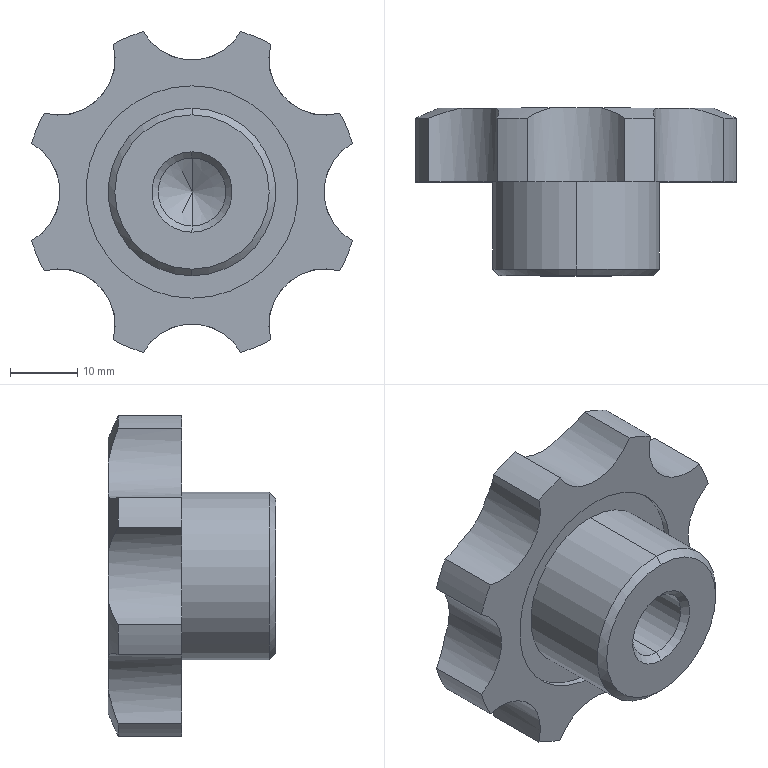Part | SolidWorks | features BaseBody 1 | 1 solid | 46 faces | box 47.841 x 25 x 47.841 mm | volume 21610 mm3 | cylinder 26 | cone 14 | plane 6 | commonest cylinder face diameters 16.667 x8 50 x8 25 x4 31.667 x4 10.106 x2
STEP:
#1=CARTESIAN_POINT('',(0.,0.947,-5.053));
#2=VERTEX_POINT('',#1);
#3=CARTESIAN_POINT('',(-0.000000001,0.947,5.053));
#4=VERTEX_POINT('',#3);
#5=CARTESIAN_POINT('',(0.,0.947,0.));
#6=DIRECTION('',(0.,-1.,0.));
#7=DIRECTION('',(0.,0.,1.));
#8=AXIS2_PLACEMENT_3D('',#5,#6,#7);
#9=CIRCLE('',#8,5.053);
#10=EDGE_CURVE('',#2,#4,#9,.T.);
#11=ORIENTED_EDGE('',*,*,#10,.F.);
#12=CARTESIAN_POINT('',(0.,0.,-6.));
#13=VERTEX_POINT('',#12);
#14=CARTESIAN_POINT('',(0.,0.,-6.));
#15=DIRECTION('',(0.,-0.7071,-0.7071));
#16=VECTOR('',#15,1000.);
#17=LINE('',#14,#16);
#18=EDGE_CURVE('',#2,#13,#17,.T.);
#19=ORIENTED_EDGE('',*,*,#18,.T.);
#20=CARTESIAN_POINT('',(0.,0.,6.));
#21=VERTEX_POINT('',#20);
#22=CARTESIAN_POINT('',(0.,0.,0.));
#23=DIRECTION('',(0.,-1.,0.));
#24=DIRECTION('',(0.,0.,-1.));
#25=AXIS2_PLACEMENT_3D('',#22,#23,#24);
#26=CIRCLE('',#25,6.);
#27=EDGE_CURVE('',#13,#21,#26,.T.);
#28=ORIENTED_EDGE('',*,*,#27,.T.);
#29=CARTESIAN_POINT('',(0.,0.,6.));
#30=DIRECTION('',(0.,-0.7071,0.7071));
#31=VECTOR('',#30,1000.);
#32=LINE('',#29,#31);
#33=EDGE_CURVE('',#4,#21,#32,.T.);
#34=ORIENTED_EDGE('',*,*,#33,.F.);
#35=EDGE_LOOP('',(#11,#19,#28,#34));
#36=FACE_OUTER_BOUND('',#35,.T.);
#37=CARTESIAN_POINT('',(0.,0.,0.));
#38=DIRECTION('',(0.,-1.,0.));
#39=DIRECTION('',(0.,0.,1.));
#40=AXIS2_PLACEMENT_3D('',#37,#38,#39);
#41=CONICAL_SURFACE('',#40,6.,0.7854);
#42=ADVANCED_FACE('',(#36),#41,.F.);
#43=CARTESIAN_POINT('',(0.,15.047,-5.053));
#44=VERTEX_POINT('',#43);
#45=CARTESIAN_POINT('',(0.,15.047,5.053));
#46=VERTEX_POINT('',#45);
#47=CARTESIAN_POINT('',(0.,15.047,0.));
#48=DIRECTION('',(0.,-1.,0.));
#49=DIRECTION('',(0.,0.,1.));
#50=AXIS2_PLACEMENT_3D('',#47,#48,#49);
#51=CIRCLE('',#50,5.053);
#52=EDGE_CURVE('',#44,#46,#51,.T.);
#53=ORIENTED_EDGE('',*,*,#52,.F.);
#54=CARTESIAN_POINT('',(0.,0.,-5.053));
#55=DIRECTION('',(0.,-1.,0.));
#56=VECTOR('',#55,1000.);
#57=LINE('',#54,#56);
#58=EDGE_CURVE('',#44,#2,#57,.T.);
#59=ORIENTED_EDGE('',*,*,#58,.T.);
#60=ORIENTED_EDGE('',*,*,#10,.T.);
#61=CARTESIAN_POINT('',(0.,0.,5.053));
#62=DIRECTION('',(0.,-1.,0.));
#63=VECTOR('',#62,1000.);
#64=LINE('',#61,#63);
#65=EDGE_CURVE('',#46,#4,#64,.T.);
#66=ORIENTED_EDGE('',*,*,#65,.F.);
#67=EDGE_LOOP('',(#53,#59,#60,#66));
#68=FACE_OUTER_BOUND('',#67,.T.);
#69=CARTESIAN_POINT('',(0.,0.,0.));
#70=DIRECTION('',(0.,-1.,0.));
#71=DIRECTION('',(0.,0.,1.));
#72=AXIS2_PLACEMENT_3D('',#69,#70,#71);
#73=CYLINDRICAL_SURFACE('',#72,5.053);
#74=ADVANCED_FACE('',(#68),#73,.F.);
#75=CARTESIAN_POINT('',(0.,17.964,0.));
#76=VERTEX_POINT('',#75);
#77=CARTESIAN_POINT('',(0.,15.047,5.053));
#78=DIRECTION('',(0.,-0.5,0.866));
#79=VECTOR('',#78,1000.);
#80=LINE('',#77,#79);
#81=EDGE_CURVE('',#76,#46,#80,.T.);
#82=ORIENTED_EDGE('',*,*,#81,.F.);
#83=CARTESIAN_POINT('',(0.,15.047,-5.053));
#84=DIRECTION('',(0.,-0.5,-0.866));
#85=VECTOR('',#84,1000.);
#86=LINE('',#83,#85);
#87=EDGE_CURVE('',#76,#44,#86,.T.);
#88=ORIENTED_EDGE('',*,*,#87,.T.);
#89=ORIENTED_EDGE('',*,*,#52,.T.);
#90=EDGE_LOOP('',(#82,#88,#89));
#91=FACE_OUTER_BOUND('',#90,.T.);
#92=CARTESIAN_POINT('',(0.,15.047,0.));
#93=DIRECTION('',(0.,-1.,0.));
#94=DIRECTION('',(0.,0.,1.));
#95=AXIS2_PLACEMENT_3D('',#92,#93,#94);
#96=CONICAL_SURFACE('',#95,5.053,1.047);
#97=ADVANCED_FACE('',(#91),#96,.F.);
#98=CARTESIAN_POINT('',(0.,0.,11.5));
#99=VERTEX_POINT('',#98);
#100=CARTESIAN_POINT('',(0.,0.,-11.5));
#101=VERTEX_POINT('',#100);
#102=CARTESIAN_POINT('',(0.,0.,0.));
#103=DIRECTION('',(0.,-1.,0.));
#104=DIRECTION('',(0.,0.,1.));
#105=AXIS2_PLACEMENT_3D('',#102,#103,#104);
#106=CIRCLE('',#105,11.5);
#107=EDGE_CURVE('',#99,#101,#106,.T.);
#108=ORIENTED_EDGE('',*,*,#107,.F.);
#109=CARTESIAN_POINT('',(0.000000015,1.,12.5));
#110=VERTEX_POINT('',#109);
#111=CARTESIAN_POINT('',(0.,1.,12.5));
#112=DIRECTION('',(0.,0.7071,0.7071));
#113=VECTOR('',#112,1000.);
#114=LINE('',#111,#113);
#115=EDGE_CURVE('',#99,#110,#114,.T.);
#116=ORIENTED_EDGE('',*,*,#115,.T.);
#117=CARTESIAN_POINT('',(-0.000000015,1.,-12.5));
#118=VERTEX_POINT('',#117);
#119=CARTESIAN_POINT('',(0.,1.,0.));
#120=DIRECTION('',(0.,-1.,0.));
#121=DIRECTION('',(0.,0.,-1.));
#122=AXIS2_PLACEMENT_3D('',#119,#120,#121);
#123=CIRCLE('',#122,12.5);
#124=EDGE_CURVE('',#110,#118,#123,.T.);
#125=ORIENTED_EDGE('',*,*,#124,.T.);
#126=CARTESIAN_POINT('',(0.,1.,-12.5));
#127=DIRECTION('',(0.,0.7071,-0.7071));
#128=VECTOR('',#127,1000.);
#129=LINE('',#126,#128);
#130=EDGE_CURVE('',#101,#118,#129,.T.);
#131=ORIENTED_EDGE('',*,*,#130,.F.);
#132=EDGE_LOOP('',(#108,#116,#125,#131));
#133=FACE_OUTER_BOUND('',#132,.T.);
#134=CARTESIAN_POINT('',(0.,1.,0.));
#135=DIRECTION('',(0.,1.,0.));
#136=DIRECTION('',(0.,0.,-1.));
#137=AXIS2_PLACEMENT_3D('',#134,#135,#136);
#138=CONICAL_SURFACE('',#137,12.5,0.7854);
#139=ADVANCED_FACE('',(#133),#138,.T.);
#140=CARTESIAN_POINT('',(0.000000015,15.,12.5));
#141=VERTEX_POINT('',#140);
#142=CARTESIAN_POINT('',(-0.000000015,15.,-12.5));
#143=VERTEX_POINT('',#142);
#144=CARTESIAN_POINT('',(0.,15.,0.));
#145=DIRECTION('',(0.,-1.,0.));
#146=DIRECTION('',(0.,0.,-1.));
#147=AXIS2_PLACEMENT_3D('',#144,#145,#146);
#148=CIRCLE('',#147,12.5);
#149=EDGE_CURVE('',#141,#143,#148,.T.);
#150=ORIENTED_EDGE('',*,*,#149,.T.);
#151=CARTESIAN_POINT('',(-0.000000015,0.,-12.5));
#152=DIRECTION('',(0.,-1.,0.));
#153=VECTOR('',#152,1000.);
#154=LINE('',#151,#153);
#155=EDGE_CURVE('',#143,#118,#154,.T.);
#156=ORIENTED_EDGE('',*,*,#155,.T.);
#157=ORIENTED_EDGE('',*,*,#124,.F.);
#158=CARTESIAN_POINT('',(0.000000015,0.,12.5));
#159=DIRECTION('',(0.,-1.,0.));
#160=VECTOR('',#159,1000.);
#161=LINE('',#158,#160);
#162=EDGE_CURVE('',#141,#110,#161,.T.);
#163=ORIENTED_EDGE('',*,*,#162,.F.);
#164=EDGE_LOOP('',(#150,#156,#157,#163));
#165=FACE_OUTER_BOUND('',#164,.T.);
#166=CARTESIAN_POINT('',(0.,0.,0.));
#167=DIRECTION('',(0.,-1.,0.));
#168=DIRECTION('',(0.000000001,0.,1.));
#169=AXIS2_PLACEMENT_3D('',#166,#167,#168);
#170=CYLINDRICAL_SURFACE('',#169,12.5);
#171=ADVANCED_FACE('',(#165),#170,.T.);
#172=CARTESIAN_POINT('',(0.,15.,-15.833));
#173=VERTEX_POINT('',#172);
#174=CARTESIAN_POINT('',(0.,15.,15.833));
#175=VERTEX_POINT('',#174);
#176=CARTESIAN_POINT('',(0.,15.,0.));
#177=DIRECTION('',(0.,-1.,0.));
#178=DIRECTION('',(0.,0.,1.));
#179=AXIS2_PLACEMENT_3D('',#176,#177,#178);
#180=CIRCLE('',#179,15.833);
#181=EDGE_CURVE('',#173,#175,#180,.T.);
#182=ORIENTED_EDGE('',*,*,#181,.F.);
#183=CARTESIAN_POINT('',(0.,14.,-15.833));
#184=VERTEX_POINT('',#183);
#185=CARTESIAN_POINT('',(0.,0.,-15.833));
#186=DIRECTION('',(0.,-1.,0.));
#187=VECTOR('',#186,1000.);
#188=LINE('',#185,#187);
#189=EDGE_CURVE('',#173,#184,#188,.T.);
#190=ORIENTED_EDGE('',*,*,#189,.T.);
#191=CARTESIAN_POINT('',(0.,14.,15.833));
#192=VERTEX_POINT('',#191);
#193=CARTESIAN_POINT('',(0.,14.,0.));
#194=DIRECTION('',(0.,-1.,0.));
#195=DIRECTION('',(0.,0.,-1.));
#196=AXIS2_PLACEMENT_3D('',#193,#194,#195);
#197=CIRCLE('',#196,15.833);
#198=EDGE_CURVE('',#184,#192,#197,.T.);
#199=ORIENTED_EDGE('',*,*,#198,.T.);
#200=CARTESIAN_POINT('',(0.,0.,15.833));
#201=DIRECTION('',(0.,-1.,0.));
#202=VECTOR('',#201,1000.);
#203=LINE('',#200,#202);
#204=EDGE_CURVE('',#175,#192,#203,.T.);
#205=ORIENTED_EDGE('',*,*,#204,.F.);
#206=EDGE_LOOP('',(#182,#190,#199,#205));
#207=FACE_OUTER_BOUND('',#206,.T.);
#208=CARTESIAN_POINT('',(0.,0.,0.));
#209=DIRECTION('',(0.,-1.,0.));
#210=DIRECTION('',(0.,0.,1.));
#211=AXIS2_PLACEMENT_3D('',#208,#209,#210);
#212=CYLINDRICAL_SURFACE('',#211,15.833);
#213=ADVANCED_FACE('',(#207),#212,.F.);
#214=CARTESIAN_POINT('',(0.,25.,-15.833));
#215=VERTEX_POINT('',#214);
#216=CARTESIAN_POINT('',(0.,25.,15.833));
#217=VERTEX_POINT('',#216);
#218=CARTESIAN_POINT('',(0.,25.,0.));
#219=DIRECTION('',(0.,-1.,0.));
#220=DIRECTION('',(0.,0.,1.));
#221=AXIS2_PLACEMENT_3D('',#218,#219,#220);
#222=CIRCLE('',#221,15.833);
#223=EDGE_CURVE('',#215,#217,#222,.T.);
#224=ORIENTED_EDGE('',*,*,#223,.F.);
#225=CARTESIAN_POINT('',(0.,24.,-15.833));
#226=VERTEX_POINT('',#225);
#227=CARTESIAN_POINT('',(0.,0.,-15.833));
#228=DIRECTION('',(0.,-1.,0.));
#229=VECTOR('',#228,1000.);
#230=LINE('',#227,#229);
#231=EDGE_CURVE('',#215,#226,#230,.T.);
#232=ORIENTED_EDGE('',*,*,#231,.T.);
#233=CARTESIAN_POINT('',(0.,24.,15.833));
#234=VERTEX_POINT('',#233);
#235=CARTESIAN_POINT('',(0.,24.,0.));
#236=DIRECTION('',(0.,-1.,0.));
#237=DIRECTION('',(0.,0.,-1.));
#238=AXIS2_PLACEMENT_3D('',#235,#236,#237);
#239=CIRCLE('',#238,15.833);
#240=EDGE_CURVE('',#226,#234,#239,.T.);
#241=ORIENTED_EDGE('',*,*,#240,.T.);
#242=CARTESIAN_POINT('',(0.,0.,15.833));
#243=DIRECTION('',(0.,-1.,0.));
#244=VECTOR('',#243,1000.);
#245=LINE('',#242,#244);
#246=EDGE_CURVE('',#217,#234,#245,.T.);
#247=ORIENTED_EDGE('',*,*,#246,.F.);
#248=EDGE_LOOP('',(#224,#232,#241,#247));
#249=FACE_OUTER_BOUND('',#248,.T.);
#250=CARTESIAN_POINT('',(0.,0.,0.));
#251=DIRECTION('',(0.,-1.,0.));
#252=DIRECTION('',(0.,0.,1.));
#253=AXIS2_PLACEMENT_3D('',#250,#251,#252);
#254=CYLINDRICAL_SURFACE('',#253,15.833);
#255=ADVANCED_FACE('',(#249),#254,.F.);
#256=CARTESIAN_POINT('',(0.,25.,12.5));
#257=VERTEX_POINT('',#256);
#258=CARTESIAN_POINT('',(0.,25.,-12.5));
#259=VERTEX_POINT('',#258);
#260=CARTESIAN_POINT('',(0.,25.,0.));
#261=DIRECTION('',(0.,-1.,0.));
#262=DIRECTION('',(0.,0.,-1.));
#263=AXIS2_PLACEMENT_3D('',#260,#261,#262);
#264=CIRCLE('',#263,12.5);
#265=EDGE_CURVE('',#257,#259,#264,.T.);
#266=ORIENTED_EDGE('',*,*,#265,.T.);
#267=CARTESIAN_POINT('',(0.,24.,-12.5));
#268=VERTEX_POINT('',#267);
#269=CARTESIAN_POINT('',(0.,0.,-12.5));
#270=DIRECTION('',(0.,-1.,0.));
#271=VECTOR('',#270,1000.);
#272=LINE('',#269,#271);
#273=EDGE_CURVE('',#259,#268,#272,.T.);
#274=ORIENTED_EDGE('',*,*,#273,.T.);
#275=CARTESIAN_POINT('',(-0.000000015,24.,12.5));
#276=VERTEX_POINT('',#275);
#277=CARTESIAN_POINT('',(0.,24.,0.));
#278=DIRECTION('',(0.,-1.,0.));
#279=DIRECTION('',(-0.000000001,0.,1.));
#280=AXIS2_PLACEMENT_3D('',#277,#278,#279);
#281=CIRCLE('',#280,12.5);
#282=EDGE_CURVE('',#276,#268,#281,.T.);
#283=ORIENTED_EDGE('',*,*,#282,.F.);
#284=CARTESIAN_POINT('',(0.,0.,12.5));
#285=DIRECTION('',(0.,-1.,0.));
#286=VECTOR('',#285,1000.);
#287=LINE('',#284,#286);
#288=EDGE_CURVE('',#257,#276,#287,.T.);
#289=ORIENTED_EDGE('',*,*,#288,.F.);
#290=EDGE_LOOP('',(#266,#274,#283,#289));
#291=FACE_OUTER_BOUND('',#290,.T.);
#292=CARTESIAN_POINT('',(0.,0.,0.));
#293=DIRECTION('',(0.,-1.,0.));
#294=DIRECTION('',(0.,0.,1.));
#295=AXIS2_PLACEMENT_3D('',#292,#293,#294);
#296=CYLINDRICAL_SURFACE('',#295,12.5);
#297=ADVANCED_FACE('',(#291),#296,.T.);
#298=CARTESIAN_POINT('',(-11.895,25.,-17.159));
#299=VERTEX_POINT('',#298);
#300=CARTESIAN_POINT('',(-11.776,23.5,-22.053));
#301=VERTEX_POINT('',#300);
#302=CARTESIAN_POINT('',(-11.895,25.,-17.159));
#303=CARTESIAN_POINT('',(-11.631,24.818,-17.949));
#304=CARTESIAN_POINT('',(-11.486,24.587,-18.784));
#305=CARTESIAN_POINT('',(-11.449,24.071,-20.447));
#306=CARTESIAN_POINT('',(-11.558,23.787,-21.275));
#307=CARTESIAN_POINT('',(-11.776,23.5,-22.053));
#308=B_SPLINE_CURVE_WITH_KNOTS('',3,(#302,#303,#304,#305,#306,#307),.UNSPECIFIED.,.F.,.F.,(4,2,4),(0.,0.5,1.),.UNSPECIFIED.);
#309=EDGE_CURVE('',#299,#301,#308,.T.);
#310=ORIENTED_EDGE('',*,*,#309,.F.);
#311=CARTESIAN_POINT('',(-3.722,25.,-20.544));
#312=VERTEX_POINT('',#311);
#313=CARTESIAN_POINT('',(0.,25.,0.));
#314=DIRECTION('',(0.,-1.,0.));
#315=DIRECTION('',(-0.5697,0.,-0.8218));
#316=AXIS2_PLACEMENT_3D('',#313,#314,#315);
#317=CIRCLE('',#316,20.879);
#318=EDGE_CURVE('',#299,#312,#317,.T.);
#319=ORIENTED_EDGE('',*,*,#318,.T.);
#320=CARTESIAN_POINT('',(-7.267,23.5,-23.921));
#321=VERTEX_POINT('',#320);
#322=CARTESIAN_POINT('',(-7.267,23.5,-23.921));
#323=CARTESIAN_POINT('',(-6.875,23.784,-23.223));
#324=CARTESIAN_POINT('',(-6.369,24.068,-22.562));
#325=CARTESIAN_POINT('',(-5.167,24.585,-21.409));
#326=CARTESIAN_POINT('',(-4.471,24.818,-20.918));
#327=CARTESIAN_POINT('',(-3.722,25.,-20.544));
#328=B_SPLINE_CURVE_WITH_KNOTS('',3,(#322,#323,#324,#325,#326,#327),.UNSPECIFIED.,.F.,.F.,(4,2,4),(0.,0.5,1.),.UNSPECIFIED.);
#329=EDGE_CURVE('',#321,#312,#328,.T.);
#330=ORIENTED_EDGE('',*,*,#329,.F.);
#331=CARTESIAN_POINT('',(0.,23.5,0.));
#332=DIRECTION('',(0.,-1.,0.));
#333=DIRECTION('',(-0.2907,0.,-0.9568));
#334=AXIS2_PLACEMENT_3D('',#331,#332,#333);
#335=CIRCLE('',#334,25.);
#336=EDGE_CURVE('',#301,#321,#335,.T.);
#337=ORIENTED_EDGE('',*,*,#336,.F.);
#338=EDGE_LOOP('',(#310,#319,#330,#337));
#339=FACE_OUTER_BOUND('',#338,.T.);
#340=CARTESIAN_POINT('',(0.,23.5,0.));
#341=DIRECTION('',(0.,-1.,0.));
#342=DIRECTION('',(-0.5697,0.,-0.8218));
#343=AXIS2_PLACEMENT_3D('',#340,#341,#342);
#344=CONICAL_SURFACE('',#343,25.,1.222);
#345=ADVANCED_FACE('',(#339),#344,.T.);
#346=CARTESIAN_POINT('',(-22.053,23.5,-11.776));
#347=VERTEX_POINT('',#346);
#348=CARTESIAN_POINT('',(-17.159,25.,-11.895));
#349=VERTEX_POINT('',#348);
#350=CARTESIAN_POINT('',(-22.053,23.5,-11.776));
#351=CARTESIAN_POINT('',(-21.283,23.784,-11.56));
#352=CARTESIAN_POINT('',(-20.457,24.068,-11.45));
#353=CARTESIAN_POINT('',(-18.792,24.585,-11.485));
#354=CARTESIAN_POINT('',(-17.953,24.818,-11.63));
#355=CARTESIAN_POINT('',(-17.159,25.,-11.895));
#356=B_SPLINE_CURVE_WITH_KNOTS('',3,(#350,#351,#352,#353,#354,#355),.UNSPECIFIED.,.F.,.F.,(4,2,4),(0.,0.5,1.),.UNSPECIFIED.);
#357=EDGE_CURVE('',#347,#349,#356,.T.);
#358=ORIENTED_EDGE('',*,*,#357,.F.);
#359=CARTESIAN_POINT('',(-23.921,23.5,-7.267));
#360=VERTEX_POINT('',#359);
#361=CARTESIAN_POINT('',(0.,23.5,0.));
#362=DIRECTION('',(0.,-1.,0.));
#363=DIRECTION('',(-0.8821,0.,-0.471));
#364=AXIS2_PLACEMENT_3D('',#361,#362,#363);
#365=CIRCLE('',#364,25.);
#366=EDGE_CURVE('',#360,#347,#365,.T.);
#367=ORIENTED_EDGE('',*,*,#366,.F.);
#368=CARTESIAN_POINT('',(-20.544,25.,-3.722));
#369=VERTEX_POINT('',#368);
#370=CARTESIAN_POINT('',(-20.544,25.,-3.722));
#371=CARTESIAN_POINT('',(-20.916,24.818,-4.467));
#372=CARTESIAN_POINT('',(-21.404,24.587,-5.16));
#373=CARTESIAN_POINT('',(-22.554,24.071,-6.362));
#374=CARTESIAN_POINT('',(-23.216,23.787,-6.871));
#375=CARTESIAN_POINT('',(-23.921,23.5,-7.267));
#376=B_SPLINE_CURVE_WITH_KNOTS('',3,(#370,#371,#372,#373,#374,#375),.UNSPECIFIED.,.F.,.F.,(4,2,4),(0.,0.5,1.),.UNSPECIFIED.);
#377=EDGE_CURVE('',#369,#360,#376,.T.);
#378=ORIENTED_EDGE('',*,*,#377,.F.);
#379=CARTESIAN_POINT('',(0.,25.,0.));
#380=DIRECTION('',(0.,-1.,0.));
#381=DIRECTION('',(-0.984,0.,-0.1783));
#382=AXIS2_PLACEMENT_3D('',#379,#380,#381);
#383=CIRCLE('',#382,20.879);
#384=EDGE_CURVE('',#369,#349,#383,.T.);
#385=ORIENTED_EDGE('',*,*,#384,.T.);
#386=EDGE_LOOP('',(#358,#367,#378,#385));
#387=FACE_OUTER_BOUND('',#386,.T.);
#388=CARTESIAN_POINT('',(0.,23.5,0.));
#389=DIRECTION('',(0.,-1.,0.));
#390=DIRECTION('',(-0.984,0.,-0.1783));
#391=AXIS2_PLACEMENT_3D('',#388,#389,#390);
#392=CONICAL_SURFACE('',#391,25.,1.222);
#393=ADVANCED_FACE('',(#387),#392,.T.);
#394=CARTESIAN_POINT('',(3.722,25.,-20.544));
#395=VERTEX_POINT('',#394);
#396=CARTESIAN_POINT('',(7.267,23.5,-23.921));
#397=VERTEX_POINT('',#396);
#398=CARTESIAN_POINT('',(3.722,25.,-20.544));
#399=CARTESIAN_POINT('',(4.467,24.818,-20.916));
#400=CARTESIAN_POINT('',(5.16,24.587,-21.404));
#401=CARTESIAN_POINT('',(6.362,24.071,-22.554));
#402=CARTESIAN_POINT('',(6.871,23.787,-23.216));
#403=CARTESIAN_POINT('',(7.267,23.5,-23.921));
#404=B_SPLINE_CURVE_WITH_KNOTS('',3,(#398,#399,#400,#401,#402,#403),.UNSPECIFIED.,.F.,.F.,(4,2,4),(0.,0.5,1.),.UNSPECIFIED.);
#405=EDGE_CURVE('',#395,#397,#404,.T.);
#406=ORIENTED_EDGE('',*,*,#405,.F.);
#407=CARTESIAN_POINT('',(11.895,25.,-17.159));
#408=VERTEX_POINT('',#407);
#409=CARTESIAN_POINT('',(0.,25.,0.));
#410=DIRECTION('',(0.,-1.,0.));
#411=DIRECTION('',(0.1783,0.,-0.984));
#412=AXIS2_PLACEMENT_3D('',#409,#410,#411);
#413=CIRCLE('',#412,20.879);
#414=EDGE_CURVE('',#395,#408,#413,.T.);
#415=ORIENTED_EDGE('',*,*,#414,.T.);
#416=CARTESIAN_POINT('',(11.776,23.5,-22.053));
#417=VERTEX_POINT('',#416);
#418=CARTESIAN_POINT('',(11.776,23.5,-22.053));
#419=CARTESIAN_POINT('',(11.56,23.784,-21.283));
#420=CARTESIAN_POINT('',(11.45,24.068,-20.457));
#421=CARTESIAN_POINT('',(11.485,24.585,-18.792));
#422=CARTESIAN_POINT('',(11.63,24.818,-17.953));
#423=CARTESIAN_POINT('',(11.895,25.,-17.159));
#424=B_SPLINE_CURVE_WITH_KNOTS('',3,(#418,#419,#420,#421,#422,#423),.UNSPECIFIED.,.F.,.F.,(4,2,4),(0.,0.5,1.),.UNSPECIFIED.);
#425=EDGE_CURVE('',#417,#408,#424,.T.);
#426=ORIENTED_EDGE('',*,*,#425,.F.);
#427=CARTESIAN_POINT('',(0.,23.5,0.));
#428=DIRECTION('',(0.,-1.,0.));
#429=DIRECTION('',(0.471,0.,-0.8821));
#430=AXIS2_PLACEMENT_3D('',#427,#428,#429);
#431=CIRCLE('',#430,25.);
#432=EDGE_CURVE('',#397,#417,#431,.T.);
#433=ORIENTED_EDGE('',*,*,#432,.F.);
#434=EDGE_LOOP('',(#406,#415,#426,#433));
#435=FACE_OUTER_BOUND('',#434,.T.);
#436=CARTESIAN_POINT('',(0.,23.5,0.));
#437=DIRECTION('',(0.,-1.,0.));
#438=DIRECTION('',(0.1783,0.,-0.984));
#439=AXIS2_PLACEMENT_3D('',#436,#437,#438);
#440=CONICAL_SURFACE('',#439,25.,1.222);
#441=ADVANCED_FACE('',(#435),#440,.T.);
#442=CARTESIAN_POINT('',(17.159,25.,-11.895));
#443=VERTEX_POINT('',#442);
#444=CARTESIAN_POINT('',(22.053,23.5,-11.776));
#445=VERTEX_POINT('',#444);
#446=CARTESIAN_POINT('',(17.159,25.,-11.895));
#447=CARTESIAN_POINT('',(17.949,24.818,-11.631));
#448=CARTESIAN_POINT('',(18.784,24.587,-11.486));
#449=CARTESIAN_POINT('',(20.447,24.071,-11.449));
#450=CARTESIAN_POINT('',(21.275,23.787,-11.558));
#451=CARTESIAN_POINT('',(22.053,23.5,-11.776));
#452=B_SPLINE_CURVE_WITH_KNOTS('',3,(#446,#447,#448,#449,#450,#451),.UNSPECIFIED.,.F.,.F.,(4,2,4),(0.,0.5,1.),.UNSPECIFIED.);
#453=EDGE_CURVE('',#443,#445,#452,.T.);
#454=ORIENTED_EDGE('',*,*,#453,.F.);
#455=CARTESIAN_POINT('',(20.544,25.,-3.722));
#456=VERTEX_POINT('',#455);
#457=CARTESIAN_POINT('',(0.,25.,0.));
#458=DIRECTION('',(0.,-1.,0.));
#459=DIRECTION('',(0.8218,0.,-0.5697));
#460=AXIS2_PLACEMENT_3D('',#457,#458,#459);
#461=CIRCLE('',#460,20.879);
#462=EDGE_CURVE('',#443,#456,#461,.T.);
#463=ORIENTED_EDGE('',*,*,#462,.T.);
#464=CARTESIAN_POINT('',(23.921,23.5,-7.267));
#465=VERTEX_POINT('',#464);
#466=CARTESIAN_POINT('',(23.921,23.5,-7.267));
#467=CARTESIAN_POINT('',(23.223,23.784,-6.875));
#468=CARTESIAN_POINT('',(22.562,24.068,-6.369));
#469=CARTESIAN_POINT('',(21.409,24.585,-5.167));
#470=CARTESIAN_POINT('',(20.918,24.818,-4.471));
#471=CARTESIAN_POINT('',(20.544,25.,-3.722));
#472=B_SPLINE_CURVE_WITH_KNOTS('',3,(#466,#467,#468,#469,#470,#471),.UNSPECIFIED.,.F.,.F.,(4,2,4),(0.,0.5,1.),.UNSPECIFIED.);
#473=EDGE_CURVE('',#465,#456,#472,.T.);
#474=ORIENTED_EDGE('',*,*,#473,.F.);
#475=CARTESIAN_POINT('',(0.,23.5,0.));
#476=DIRECTION('',(0.,-1.,0.));
#477=DIRECTION('',(0.9568,0.,-0.2907));
#478=AXIS2_PLACEMENT_3D('',#475,#476,#477);
#479=CIRCLE('',#478,25.);
#480=EDGE_CURVE('',#445,#465,#479,.T.);
#481=ORIENTED_EDGE('',*,*,#480,.F.);
#482=EDGE_LOOP('',(#454,#463,#474,#481));
#483=FACE_OUTER_BOUND('',#482,.T.);
#484=CARTESIAN_POINT('',(0.,23.5,0.));
#485=DIRECTION('',(0.,-1.,0.));
#486=DIRECTION('',(0.8218,0.,-0.5697));
#487=AXIS2_PLACEMENT_3D('',#484,#485,#486);
#488=CONICAL_SURFACE('',#487,25.,1.222);
#489=ADVANCED_FACE('',(#483),#488,.T.);
#490=CARTESIAN_POINT('',(20.544,25.,3.722));
#491=VERTEX_POINT('',#490);
#492=CARTESIAN_POINT('',(23.921,23.5,7.267));
#493=VERTEX_POINT('',#492);
#494=CARTESIAN_POINT('',(20.544,25.,3.722));
#495=CARTESIAN_POINT('',(20.916,24.818,4.467));
#496=CARTESIAN_POINT('',(21.404,24.587,5.16));
#497=CARTESIAN_POINT('',(22.554,24.071,6.362));
#498=CARTESIAN_POINT('',(23.216,23.787,6.871));
#499=CARTESIAN_POINT('',(23.921,23.5,7.267));
#500=B_SPLINE_CURVE_WITH_KNOTS('',3,(#494,#495,#496,#497,#498,#499),.UNSPECIFIED.,.F.,.F.,(4,2,4),(0.,0.5,1.),.UNSPECIFIED.);
#501=EDGE_CURVE('',#491,#493,#500,.T.);
#502=ORIENTED_EDGE('',*,*,#501,.F.);
#503=CARTESIAN_POINT('',(17.159,25.,11.895));
#504=VERTEX_POINT('',#503);
#505=CARTESIAN_POINT('',(0.,25.,0.));
#506=DIRECTION('',(0.,-1.,0.));
#507=DIRECTION('',(0.984,0.,0.1783));
#508=AXIS2_PLACEMENT_3D('',#505,#506,#507);
#509=CIRCLE('',#508,20.879);
#510=EDGE_CURVE('',#491,#504,#509,.T.);
#511=ORIENTED_EDGE('',*,*,#510,.T.);
#512=CARTESIAN_POINT('',(22.053,23.5,11.776));
#513=VERTEX_POINT('',#512);
#514=CARTESIAN_POINT('',(22.053,23.5,11.776));
#515=CARTESIAN_POINT('',(21.283,23.784,11.56));
#516=CARTESIAN_POINT('',(20.457,24.068,11.45));
#517=CARTESIAN_POINT('',(18.792,24.585,11.485));
#518=CARTESIAN_POINT('',(17.953,24.818,11.63));
#519=CARTESIAN_POINT('',(17.159,25.,11.895));
#520=B_SPLINE_CURVE_WITH_KNOTS('',3,(#514,#515,#516,#517,#518,#519),.UNSPECIFIED.,.F.,.F.,(4,2,4),(0.,0.5,1.),.UNSPECIFIED.);
#521=EDGE_CURVE('',#513,#504,#520,.T.);
#522=ORIENTED_EDGE('',*,*,#521,.F.);
#523=CARTESIAN_POINT('',(0.,23.5,0.));
#524=DIRECTION('',(0.,-1.,0.));
#525=DIRECTION('',(0.8821,0.,0.471));
#526=AXIS2_PLACEMENT_3D('',#523,#524,#525);
#527=CIRCLE('',#526,25.);
#528=EDGE_CURVE('',#493,#513,#527,.T.);
#529=ORIENTED_EDGE('',*,*,#528,.F.);
#530=EDGE_LOOP('',(#502,#511,#522,#529));
#531=FACE_OUTER_BOUND('',#530,.T.);
#532=CARTESIAN_POINT('',(0.,23.5,0.));
#533=DIRECTION('',(0.,-1.,0.));
#534=DIRECTION('',(0.984,0.,0.1783));
#535=AXIS2_PLACEMENT_3D('',#532,#533,#534);
#536=CONICAL_SURFACE('',#535,25.,1.222);
#537=ADVANCED_FACE('',(#531),#536,.T.);
#538=CARTESIAN_POINT('',(11.895,25.,17.159));
#539=VERTEX_POINT('',#538);
#540=CARTESIAN_POINT('',(11.776,23.5,22.053));
#541=VERTEX_POINT('',#540);
#542=CARTESIAN_POINT('',(11.895,25.,17.159));
#543=CARTESIAN_POINT('',(11.631,24.818,17.949));
#544=CARTESIAN_POINT('',(11.486,24.587,18.784));
#545=CARTESIAN_POINT('',(11.449,24.071,20.447));
#546=CARTESIAN_POINT('',(11.558,23.787,21.275));
#547=CARTESIAN_POINT('',(11.776,23.5,22.053));
#548=B_SPLINE_CURVE_WITH_KNOTS('',3,(#542,#543,#544,#545,#546,#547),.UNSPECIFIED.,.F.,.F.,(4,2,4),(0.,0.5,1.),.UNSPECIFIED.);
#549=EDGE_CURVE('',#539,#541,#548,.T.);
#550=ORIENTED_EDGE('',*,*,#549,.F.);
#551=CARTESIAN_POINT('',(3.722,25.,20.544));
#552=VERTEX_POINT('',#551);
#553=CARTESIAN_POINT('',(0.,25.,0.));
#554=DIRECTION('',(0.,-1.,0.));
#555=DIRECTION('',(0.5697,0.,0.8218));
#556=AXIS2_PLACEMENT_3D('',#553,#554,#555);
#557=CIRCLE('',#556,20.879);
#558=EDGE_CURVE('',#539,#552,#557,.T.);
#559=ORIENTED_EDGE('',*,*,#558,.T.);
#560=CARTESIAN_POINT('',(7.267,23.5,23.921));
#561=VERTEX_POINT('',#560);
#562=CARTESIAN_POINT('',(7.267,23.5,23.921));
#563=CARTESIAN_POINT('',(6.875,23.784,23.223));
#564=CARTESIAN_POINT('',(6.369,24.068,22.562));
#565=CARTESIAN_POINT('',(5.167,24.585,21.409));
#566=CARTESIAN_POINT('',(4.471,24.818,20.918));
#567=CARTESIAN_POINT('',(3.722,25.,20.544));
#568=B_SPLINE_CURVE_WITH_KNOTS('',3,(#562,#563,#564,#565,#566,#567),.UNSPECIFIED.,.F.,.F.,(4,2,4),(0.,0.5,1.),.UNSPECIFIED.);
#569=EDGE_CURVE('',#561,#552,#568,.T.);
#570=ORIENTED_EDGE('',*,*,#569,.F.);
#571=CARTESIAN_POINT('',(0.,23.5,0.));
#572=DIRECTION('',(0.,-1.,0.));
#573=DIRECTION('',(0.2907,0.,0.9568));
#574=AXIS2_PLACEMENT_3D('',#571,#572,#573);
#575=CIRCLE('',#574,25.);
#576=EDGE_CURVE('',#541,#561,#575,.T.);
#577=ORIENTED_EDGE('',*,*,#576,.F.);
#578=EDGE_LOOP('',(#550,#559,#570,#577));
#579=FACE_OUTER_BOUND('',#578,.T.);
#580=CARTESIAN_POINT('',(0.,23.5,0.));
#581=DIRECTION('',(0.,-1.,0.));
#582=DIRECTION('',(0.5697,0.,0.8218));
#583=AXIS2_PLACEMENT_3D('',#580,#581,#582);
#584=CONICAL_SURFACE('',#583,25.,1.222);
#585=ADVANCED_FACE('',(#579),#584,.T.);
#586=CARTESIAN_POINT('',(-3.722,25.,20.544));
#587=VERTEX_POINT('',#586);
#588=CARTESIAN_POINT('',(-7.267,23.5,23.921));
#589=VERTEX_POINT('',#588);
#590=CARTESIAN_POINT('',(-3.722,25.,20.544));
#591=CARTESIAN_POINT('',(-4.467,24.818,20.916));
#592=CARTESIAN_POINT('',(-5.16,24.587,21.404));
#593=CARTESIAN_POINT('',(-6.362,24.071,22.554));
#594=CARTESIAN_POINT('',(-6.871,23.787,23.216));
#595=CARTESIAN_POINT('',(-7.267,23.5,23.921));
#596=B_SPLINE_CURVE_WITH_KNOTS('',3,(#590,#591,#592,#593,#594,#595),.UNSPECIFIED.,.F.,.F.,(4,2,4),(0.,0.5,1.),.UNSPECIFIED.);
#597=EDGE_CURVE('',#587,#589,#596,.T.);
#598=ORIENTED_EDGE('',*,*,#597,.F.);
#599=CARTESIAN_POINT('',(-11.895,25.,17.159));
#600=VERTEX_POINT('',#599);
#601=CARTESIAN_POINT('',(0.,25.,0.));
#602=DIRECTION('',(0.,-1.,0.));
#603=DIRECTION('',(-0.1783,0.,0.984));
#604=AXIS2_PLACEMENT_3D('',#601,#602,#603);
#605=CIRCLE('',#604,20.879);
#606=EDGE_CURVE('',#587,#600,#605,.T.);
#607=ORIENTED_EDGE('',*,*,#606,.T.);
#608=CARTESIAN_POINT('',(-11.776,23.5,22.053));
#609=VERTEX_POINT('',#608);
#610=CARTESIAN_POINT('',(-11.776,23.5,22.053));
#611=CARTESIAN_POINT('',(-11.56,23.784,21.283));
#612=CARTESIAN_POINT('',(-11.45,24.068,20.457));
#613=CARTESIAN_POINT('',(-11.485,24.585,18.792));
#614=CARTESIAN_POINT('',(-11.63,24.818,17.953));
#615=CARTESIAN_POINT('',(-11.895,25.,17.159));
#616=B_SPLINE_CURVE_WITH_KNOTS('',3,(#610,#611,#612,#613,#614,#615),.UNSPECIFIED.,.F.,.F.,(4,2,4),(0.,0.5,1.),.UNSPECIFIED.);
#617=EDGE_CURVE('',#609,#600,#616,.T.);
#618=ORIENTED_EDGE('',*,*,#617,.F.);
#619=CARTESIAN_POINT('',(0.,23.5,0.));
#620=DIRECTION('',(0.,-1.,0.));
#621=DIRECTION('',(-0.471,0.,0.8821));
#622=AXIS2_PLACEMENT_3D('',#619,#620,#621);
#623=CIRCLE('',#622,25.);
#624=EDGE_CURVE('',#589,#609,#623,.T.);
#625=ORIENTED_EDGE('',*,*,#624,.F.);
#626=EDGE_LOOP('',(#598,#607,#618,#625));
#627=FACE_OUTER_BOUND('',#626,.T.);
#628=CARTESIAN_POINT('',(0.,23.5,0.));
#629=DIRECTION('',(0.,-1.,0.));
#630=DIRECTION('',(-0.1783,0.,0.984));
#631=AXIS2_PLACEMENT_3D('',#628,#629,#630);
#632=CONICAL_SURFACE('',#631,25.,1.222);
#633=ADVANCED_FACE('',(#627),#632,.T.);
#634=CARTESIAN_POINT('',(-17.159,25.,11.895));
#635=VERTEX_POINT('',#634);
#636=CARTESIAN_POINT('',(-22.053,23.5,11.776));
#637=VERTEX_POINT('',#636);
#638=CARTESIAN_POINT('',(-17.159,25.,11.895));
#639=CARTESIAN_POINT('',(-17.949,24.818,11.631));
#640=CARTESIAN_POINT('',(-18.784,24.587,11.486));
#641=CARTESIAN_POINT('',(-20.447,24.071,11.449));
#642=CARTESIAN_POINT('',(-21.275,23.787,11.558));
#643=CARTESIAN_POINT('',(-22.053,23.5,11.776));
#644=B_SPLINE_CURVE_WITH_KNOTS('',3,(#638,#639,#640,#641,#642,#643),.UNSPECIFIED.,.F.,.F.,(4,2,4),(0.,0.5,1.),.UNSPECIFIED.);
#645=EDGE_CURVE('',#635,#637,#644,.T.);
#646=ORIENTED_EDGE('',*,*,#645,.F.);
#647=CARTESIAN_POINT('',(-20.544,25.,3.722));
#648=VERTEX_POINT('',#647);
#649=CARTESIAN_POINT('',(0.,25.,0.));
#650=DIRECTION('',(0.,-1.,0.));
#651=DIRECTION('',(-0.8218,0.,0.5697));
#652=AXIS2_PLACEMENT_3D('',#649,#650,#651);
#653=CIRCLE('',#652,20.879);
#654=EDGE_CURVE('',#635,#648,#653,.T.);
#655=ORIENTED_EDGE('',*,*,#654,.T.);
#656=CARTESIAN_POINT('',(-23.921,23.5,7.267));
#657=VERTEX_POINT('',#656);
#658=CARTESIAN_POINT('',(-23.921,23.5,7.267));
#659=CARTESIAN_POINT('',(-23.223,23.784,6.875));
#660=CARTESIAN_POINT('',(-22.562,24.068,6.369));
#661=CARTESIAN_POINT('',(-21.409,24.585,5.167));
#662=CARTESIAN_POINT('',(-20.918,24.818,4.471));
#663=CARTESIAN_POINT('',(-20.544,25.,3.722));
#664=B_SPLINE_CURVE_WITH_KNOTS('',3,(#658,#659,#660,#661,#662,#663),.UNSPECIFIED.,.F.,.F.,(4,2,4),(0.,0.5,1.),.UNSPECIFIED.);
#665=EDGE_CURVE('',#657,#648,#664,.T.);
#666=ORIENTED_EDGE('',*,*,#665,.F.);
#667=CARTESIAN_POINT('',(0.,23.5,0.));
#668=DIRECTION('',(0.,-1.,0.));
#669=DIRECTION('',(-0.9568,0.,0.2907));
#670=AXIS2_PLACEMENT_3D('',#667,#668,#669);
#671=CIRCLE('',#670,25.);
#672=EDGE_CURVE('',#637,#657,#671,.T.);
#673=ORIENTED_EDGE('',*,*,#672,.F.);
#674=EDGE_LOOP('',(#646,#655,#666,#673));
#675=FACE_OUTER_BOUND('',#674,.T.);
#676=CARTESIAN_POINT('',(0.,23.5,0.));
#677=DIRECTION('',(0.,-1.,0.));
#678=DIRECTION('',(-0.8218,0.,0.5697));
#679=AXIS2_PLACEMENT_3D('',#676,#677,#678);
#680=CONICAL_SURFACE('',#679,25.,1.222);
#681=ADVANCED_FACE('',(#675),#680,.T.);
#682=CARTESIAN_POINT('',(-11.776,14.,-22.053));
#683=VERTEX_POINT('',#682);
#684=CARTESIAN_POINT('',(-11.776,14.,-22.053));
#685=DIRECTION('',(0.,-1.,0.));
#686=VECTOR('',#685,1000.);
#687=LINE('',#684,#686);
#688=EDGE_CURVE('',#301,#683,#687,.T.);
#689=ORIENTED_EDGE('',*,*,#688,.F.);
#690=ORIENTED_EDGE('',*,*,#336,.T.);
#691=CARTESIAN_POINT('',(-7.267,14.,-23.921));
#692=VERTEX_POINT('',#691);
#693=CARTESIAN_POINT('',(-7.267,23.5,-23.921));
#694=DIRECTION('',(0.,-1.,0.));
#695=VECTOR('',#694,1000.);
#696=LINE('',#693,#695);
#697=EDGE_CURVE('',#321,#692,#696,.T.);
#698=ORIENTED_EDGE('',*,*,#697,.T.);
#699=CARTESIAN_POINT('',(0.,14.,0.));
#700=DIRECTION('',(0.,-1.,0.));
#701=DIRECTION('',(-0.2907,0.,-0.9568));
#702=AXIS2_PLACEMENT_3D('',#699,#700,#701);
#703=CIRCLE('',#702,25.);
#704=EDGE_CURVE('',#683,#692,#703,.T.);
#705=ORIENTED_EDGE('',*,*,#704,.F.);
#706=EDGE_LOOP('',(#689,#690,#698,#705));
#707=FACE_OUTER_BOUND('',#706,.T.);
#708=CARTESIAN_POINT('',(0.,0.,0.));
#709=DIRECTION('',(0.,-1.,0.));
#710=DIRECTION('',(-0.471,0.,-0.8821));
#711=AXIS2_PLACEMENT_3D('',#708,#709,#710);
#712=CYLINDRICAL_SURFACE('',#711,25.);
#713=ADVANCED_FACE('',(#707),#712,.T.);
#714=CARTESIAN_POINT('',(-22.053,14.,-11.776));
#715=VERTEX_POINT('',#714);
#716=CARTESIAN_POINT('',(-22.053,23.5,-11.776));
#717=DIRECTION('',(0.,-1.,0.));
#718=VECTOR('',#717,1000.);
#719=LINE('',#716,#718);
#720=EDGE_CURVE('',#347,#715,#719,.T.);
#721=ORIENTED_EDGE('',*,*,#720,.T.);
#722=CARTESIAN_POINT('',(-23.921,14.,-7.267));
#723=VERTEX_POINT('',#722);
#724=CARTESIAN_POINT('',(0.,14.,0.));
#725=DIRECTION('',(0.,-1.,0.));
#726=DIRECTION('',(-0.8821,0.,-0.471));
#727=AXIS2_PLACEMENT_3D('',#724,#725,#726);
#728=CIRCLE('',#727,25.);
#729=EDGE_CURVE('',#723,#715,#728,.T.);
#730=ORIENTED_EDGE('',*,*,#729,.F.);
#731=CARTESIAN_POINT('',(-23.921,14.,-7.267));
#732=DIRECTION('',(0.,-1.,0.));
#733=VECTOR('',#732,1000.);
#734=LINE('',#731,#733);
#735=EDGE_CURVE('',#360,#723,#734,.T.);
#736=ORIENTED_EDGE('',*,*,#735,.F.);
#737=ORIENTED_EDGE('',*,*,#366,.T.);
#738=EDGE_LOOP('',(#721,#730,#736,#737));
#739=FACE_OUTER_BOUND('',#738,.T.);
#740=CARTESIAN_POINT('',(0.,0.,0.));
#741=DIRECTION('',(0.,-1.,0.));
#742=DIRECTION('',(-0.9568,0.,-0.2907));
#743=AXIS2_PLACEMENT_3D('',#740,#741,#742);
#744=CYLINDRICAL_SURFACE('',#743,25.);
#745=ADVANCED_FACE('',(#739),#744,.T.);
#746=CARTESIAN_POINT('',(7.267,14.,-23.921));
#747=VERTEX_POINT('',#746);
#748=CARTESIAN_POINT('',(7.267,14.,-23.921));
#749=DIRECTION('',(0.,-1.,0.));
#750=VECTOR('',#749,1000.);
#751=LINE('',#748,#750);
#752=EDGE_CURVE('',#397,#747,#751,.T.);
#753=ORIENTED_EDGE('',*,*,#752,.F.);
#754=ORIENTED_EDGE('',*,*,#432,.T.);
#755=CARTESIAN_POINT('',(11.776,14.,-22.053));
#756=VERTEX_POINT('',#755);
#757=CARTESIAN_POINT('',(11.776,23.5,-22.053));
#758=DIRECTION('',(0.,-1.,0.));
#759=VECTOR('',#758,1000.);
#760=LINE('',#757,#759);
#761=EDGE_CURVE('',#417,#756,#760,.T.);
#762=ORIENTED_EDGE('',*,*,#761,.T.);
#763=CARTESIAN_POINT('',(0.,14.,0.));
#764=DIRECTION('',(0.,-1.,0.));
#765=DIRECTION('',(0.471,0.,-0.8821));
#766=AXIS2_PLACEMENT_3D('',#763,#764,#765);
#767=CIRCLE('',#766,25.);
#768=EDGE_CURVE('',#747,#756,#767,.T.);
#769=ORIENTED_EDGE('',*,*,#768,.F.);
#770=EDGE_LOOP('',(#753,#754,#762,#769));
#771=FACE_OUTER_BOUND('',#770,.T.);
#772=CARTESIAN_POINT('',(0.,0.,0.));
#773=DIRECTION('',(0.,-1.,0.));
#774=DIRECTION('',(0.2907,0.,-0.9568));
#775=AXIS2_PLACEMENT_3D('',#772,#773,#774);
#776=CYLINDRICAL_SURFACE('',#775,25.);
#777=ADVANCED_FACE('',(#771),#776,.T.);
#778=CARTESIAN_POINT('',(22.053,14.,-11.776));
#779=VERTEX_POINT('',#778);
#780=CARTESIAN_POINT('',(22.053,14.,-11.776));
#781=DIRECTION('',(0.,-1.,0.));
#782=VECTOR('',#781,1000.);
#783=LINE('',#780,#782);
#784=EDGE_CURVE('',#445,#779,#783,.T.);
#785=ORIENTED_EDGE('',*,*,#784,.F.);
#786=ORIENTED_EDGE('',*,*,#480,.T.);
#787=CARTESIAN_POINT('',(23.921,14.,-7.267));
#788=VERTEX_POINT('',#787);
#789=CARTESIAN_POINT('',(23.921,23.5,-7.267));
#790=DIRECTION('',(0.,-1.,0.));
#791=VECTOR('',#790,1000.);
#792=LINE('',#789,#791);
#793=EDGE_CURVE('',#465,#788,#792,.T.);
#794=ORIENTED_EDGE('',*,*,#793,.T.);
#795=CARTESIAN_POINT('',(0.,14.,0.));
#796=DIRECTION('',(0.,-1.,0.));
#797=DIRECTION('',(0.9568,0.,-0.2907));
#798=AXIS2_PLACEMENT_3D('',#795,#796,#797);
#799=CIRCLE('',#798,25.);
#800=EDGE_CURVE('',#779,#788,#799,.T.);
#801=ORIENTED_EDGE('',*,*,#800,.F.);
#802=EDGE_LOOP('',(#785,#786,#794,#801));
#803=FACE_OUTER_BOUND('',#802,.T.);
#804=CARTESIAN_POINT('',(0.,0.,0.));
#805=DIRECTION('',(0.,-1.,0.));
#806=DIRECTION('',(0.8821,0.,-0.471));
#807=AXIS2_PLACEMENT_3D('',#804,#805,#806);
#808=CYLINDRICAL_SURFACE('',#807,25.);
#809=ADVANCED_FACE('',(#803),#808,.T.);
#810=CARTESIAN_POINT('',(23.921,14.,7.267));
#811=VERTEX_POINT('',#810);
#812=CARTESIAN_POINT('',(23.921,14.,7.267));
#813=DIRECTION('',(0.,-1.,0.));
#814=VECTOR('',#813,1000.);
#815=LINE('',#812,#814);
#816=EDGE_CURVE('',#493,#811,#815,.T.);
#817=ORIENTED_EDGE('',*,*,#816,.F.);
#818=ORIENTED_EDGE('',*,*,#528,.T.);
#819=CARTESIAN_POINT('',(22.053,14.,11.776));
#820=VERTEX_POINT('',#819);
#821=CARTESIAN_POINT('',(22.053,23.5,11.776));
#822=DIRECTION('',(0.,-1.,0.));
#823=VECTOR('',#822,1000.);
#824=LINE('',#821,#823);
#825=EDGE_CURVE('',#513,#820,#824,.T.);
#826=ORIENTED_EDGE('',*,*,#825,.T.);
#827=CARTESIAN_POINT('',(0.,14.,0.));
#828=DIRECTION('',(0.,-1.,0.));
#829=DIRECTION('',(0.8821,0.,0.471));
#830=AXIS2_PLACEMENT_3D('',#827,#828,#829);
#831=CIRCLE('',#830,25.);
#832=EDGE_CURVE('',#811,#820,#831,.T.);
#833=ORIENTED_EDGE('',*,*,#832,.F.);
#834=EDGE_LOOP('',(#817,#818,#826,#833));
#835=FACE_OUTER_BOUND('',#834,.T.);
#836=CARTESIAN_POINT('',(0.,0.,0.));
#837=DIRECTION('',(0.,-1.,0.));
#838=DIRECTION('',(0.9568,0.,0.2907));
#839=AXIS2_PLACEMENT_3D('',#836,#837,#838);
#840=CYLINDRICAL_SURFACE('',#839,25.);
#841=ADVANCED_FACE('',(#835),#840,.T.);
#842=CARTESIAN_POINT('',(11.776,14.,22.053));
#843=VERTEX_POINT('',#842);
#844=CARTESIAN_POINT('',(11.776,14.,22.053));
#845=DIRECTION('',(0.,-1.,0.));
#846=VECTOR('',#845,1000.);
#847=LINE('',#844,#846);
#848=EDGE_CURVE('',#541,#843,#847,.T.);
#849=ORIENTED_EDGE('',*,*,#848,.F.);
#850=ORIENTED_EDGE('',*,*,#576,.T.);
#851=CARTESIAN_POINT('',(7.267,14.,23.921));
#852=VERTEX_POINT('',#851);
#853=CARTESIAN_POINT('',(7.267,23.5,23.921));
#854=DIRECTION('',(0.,-1.,0.));
#855=VECTOR('',#854,1000.);
#856=LINE('',#853,#855);
#857=EDGE_CURVE('',#561,#852,#856,.T.);
#858=ORIENTED_EDGE('',*,*,#857,.T.);
#859=CARTESIAN_POINT('',(0.,14.,0.));
#860=DIRECTION('',(0.,-1.,0.));
#861=DIRECTION('',(0.2907,0.,0.9568));
#862=AXIS2_PLACEMENT_3D('',#859,#860,#861);
#863=CIRCLE('',#862,25.);
#864=EDGE_CURVE('',#843,#852,#863,.T.);
#865=ORIENTED_EDGE('',*,*,#864,.F.);
#866=EDGE_LOOP('',(#849,#850,#858,#865));
#867=FACE_OUTER_BOUND('',#866,.T.);
#868=CARTESIAN_POINT('',(0.,0.,0.));
#869=DIRECTION('',(0.,-1.,0.));
#870=DIRECTION('',(0.471,0.,0.8821));
#871=AXIS2_PLACEMENT_3D('',#868,#869,#870);
#872=CYLINDRICAL_SURFACE('',#871,25.);
#873=ADVANCED_FACE('',(#867),#872,.T.);
#874=CARTESIAN_POINT('',(-7.267,14.,23.921));
#875=VERTEX_POINT('',#874);
#876=CARTESIAN_POINT('',(-7.267,14.,23.921));
#877=DIRECTION('',(0.,-1.,0.));
#878=VECTOR('',#877,1000.);
#879=LINE('',#876,#878);
#880=EDGE_CURVE('',#589,#875,#879,.T.);
#881=ORIENTED_EDGE('',*,*,#880,.F.);
#882=ORIENTED_EDGE('',*,*,#624,.T.);
#883=CARTESIAN_POINT('',(-11.776,14.,22.053));
#884=VERTEX_POINT('',#883);
#885=CARTESIAN_POINT('',(-11.776,23.5,22.053));
#886=DIRECTION('',(0.,-1.,0.));
#887=VECTOR('',#886,1000.);
#888=LINE('',#885,#887);
#889=EDGE_CURVE('',#609,#884,#888,.T.);
#890=ORIENTED_EDGE('',*,*,#889,.T.);
#891=CARTESIAN_POINT('',(0.,14.,0.));
#892=DIRECTION('',(0.,-1.,0.));
#893=DIRECTION('',(-0.471,0.,0.8821));
#894=AXIS2_PLACEMENT_3D('',#891,#892,#893);
#895=CIRCLE('',#894,25.);
#896=EDGE_CURVE('',#875,#884,#895,.T.);
#897=ORIENTED_EDGE('',*,*,#896,.F.);
#898=EDGE_LOOP('',(#881,#882,#890,#897));
#899=FACE_OUTER_BOUND('',#898,.T.);
#900=CARTESIAN_POINT('',(0.,0.,0.));
#901=DIRECTION('',(0.,-1.,0.));
#902=DIRECTION('',(-0.2907,0.,0.9568));
#903=AXIS2_PLACEMENT_3D('',#900,#901,#902);
#904=CYLINDRICAL_SURFACE('',#903,25.);
#905=ADVANCED_FACE('',(#899),#904,.T.);
#906=CARTESIAN_POINT('',(-22.053,14.,11.776));
#907=VERTEX_POINT('',#906);
#908=CARTESIAN_POINT('',(-22.053,14.,11.776));
#909=DIRECTION('',(0.,-1.,0.));
#910=VECTOR('',#909,1000.);
#911=LINE('',#908,#910);
#912=EDGE_CURVE('',#637,#907,#911,.T.);
#913=ORIENTED_EDGE('',*,*,#912,.F.);
#914=ORIENTED_EDGE('',*,*,#672,.T.);
#915=CARTESIAN_POINT('',(-23.921,14.,7.267));
#916=VERTEX_POINT('',#915);
#917=CARTESIAN_POINT('',(-23.921,23.5,7.267));
#918=DIRECTION('',(0.,-1.,0.));
#919=VECTOR('',#918,1000.);
#920=LINE('',#917,#919);
#921=EDGE_CURVE('',#657,#916,#920,.T.);
#922=ORIENTED_EDGE('',*,*,#921,.T.);
#923=CARTESIAN_POINT('',(0.,14.,0.));
#924=DIRECTION('',(0.,-1.,0.));
#925=DIRECTION('',(-0.9568,0.,0.2907));
#926=AXIS2_PLACEMENT_3D('',#923,#924,#925);
#927=CIRCLE('',#926,25.);
#928=EDGE_CURVE('',#907,#916,#927,.T.);
#929=ORIENTED_EDGE('',*,*,#928,.F.);
#930=EDGE_LOOP('',(#913,#914,#922,#929));
#931=FACE_OUTER_BOUND('',#930,.T.);
#932=CARTESIAN_POINT('',(0.,0.,0.));
#933=DIRECTION('',(0.,-1.,0.));
#934=DIRECTION('',(-0.8821,0.,0.471));
#935=AXIS2_PLACEMENT_3D('',#932,#933,#934);
#936=CYLINDRICAL_SURFACE('',#935,25.);
#937=ADVANCED_FACE('',(#931),#936,.T.);
#938=ORIENTED_EDGE('',*,*,#265,.F.);
#939=CARTESIAN_POINT('',(0.,25.,0.));
#940=DIRECTION('',(0.,-1.,0.));
#941=DIRECTION('',(0.,0.,-1.));
#942=AXIS2_PLACEMENT_3D('',#939,#940,#941);
#943=CIRCLE('',#942,12.5);
#944=EDGE_CURVE('',#259,#257,#943,.T.);
#945=ORIENTED_EDGE('',*,*,#944,.F.);
#946=EDGE_LOOP('',(#938,#945));
#947=FACE_OUTER_BOUND('',#946,.T.);
#948=CARTESIAN_POINT('',(-12.732,25.,12.5));
#949=DIRECTION('',(0.,1.,0.));
#950=DIRECTION('',(1.,0.,0.));
#951=AXIS2_PLACEMENT_3D('',#948,#949,#950);
#952=PLANE('',#951);
#953=ADVANCED_FACE('',(#947),#952,.T.);
#954=CARTESIAN_POINT('',(0.,24.,0.));
#955=DIRECTION('',(0.,-1.,0.));
#956=DIRECTION('',(0.,0.,-1.));
#957=AXIS2_PLACEMENT_3D('',#954,#955,#956);
#958=CIRCLE('',#957,15.833);
#959=EDGE_CURVE('',#234,#226,#958,.T.);
#960=ORIENTED_EDGE('',*,*,#959,.F.);
#961=ORIENTED_EDGE('',*,*,#240,.F.);
#962=EDGE_LOOP('',(#960,#961));
#963=FACE_OUTER_BOUND('',#962,.T.);
#964=ORIENTED_EDGE('',*,*,#282,.T.);
#965=CARTESIAN_POINT('',(0.,24.,0.));
#966=DIRECTION('',(0.,-1.,0.));
#967=DIRECTION('',(-0.000000001,0.,1.));
#968=AXIS2_PLACEMENT_3D('',#965,#966,#967);
#969=CIRCLE('',#968,12.5);
#970=EDGE_CURVE('',#268,#276,#969,.T.);
#971=ORIENTED_EDGE('',*,*,#970,.T.);
#972=EDGE_LOOP('',(#964,#971));
#973=FACE_BOUND('',#972,.T.);
#974=CARTESIAN_POINT('',(-16.127,24.,15.833));
#975=DIRECTION('',(0.,1.,0.));
#976=DIRECTION('',(1.,0.,0.));
#977=AXIS2_PLACEMENT_3D('',#974,#975,#976);
#978=PLANE('',#977);
#979=ADVANCED_FACE('',(#963,#973),#978,.T.);
#980=CARTESIAN_POINT('',(28.,25.,0.));
#981=DIRECTION('',(0.,1.,0.));
#982=DIRECTION('',(-0.8947,0.,0.4467));
#983=AXIS2_PLACEMENT_3D('',#980,#981,#982);
#984=CIRCLE('',#983,8.333);
#985=EDGE_CURVE('',#456,#491,#984,.T.);
#986=ORIENTED_EDGE('',*,*,#985,.F.);
#987=ORIENTED_EDGE('',*,*,#462,.F.);
#988=CARTESIAN_POINT('',(19.799,25.,-19.799));
#989=DIRECTION('',(0.,1.,0.));
#990=DIRECTION('',(-0.3168,0.,0.9485));
#991=AXIS2_PLACEMENT_3D('',#988,#989,#990);
#992=CIRCLE('',#991,8.333);
#993=EDGE_CURVE('',#408,#443,#992,.T.);
#994=ORIENTED_EDGE('',*,*,#993,.F.);
#995=ORIENTED_EDGE('',*,*,#414,.F.);
#996=CARTESIAN_POINT('',(0.,25.,-28.));
#997=DIRECTION('',(0.,1.,0.));
#998=DIRECTION('',(0.4467,0.,0.8947));
#999=AXIS2_PLACEMENT_3D('',#996,#997,#998);
#1000=CIRCLE('',#999,8.333);
#1001=EDGE_CURVE('',#312,#395,#1000,.T.);
#1002=ORIENTED_EDGE('',*,*,#1001,.F.);
#1003=ORIENTED_EDGE('',*,*,#318,.F.);
#1004=CARTESIAN_POINT('',(-19.799,25.,-19.799));
#1005=DIRECTION('',(0.,1.,0.));
#1006=DIRECTION('',(0.9485,0.,0.3168));
#1007=AXIS2_PLACEMENT_3D('',#1004,#1005,#1006);
#1008=CIRCLE('',#1007,8.333);
#1009=EDGE_CURVE('',#349,#299,#1008,.T.);
#1010=ORIENTED_EDGE('',*,*,#1009,.F.);
#1011=ORIENTED_EDGE('',*,*,#384,.F.);
#1012=CARTESIAN_POINT('',(-28.,25.,0.));
#1013=DIRECTION('',(0.,1.,0.));
#1014=DIRECTION('',(0.8947,0.,-0.4467));
#1015=AXIS2_PLACEMENT_3D('',#1012,#1013,#1014);
#1016=CIRCLE('',#1015,8.333);
#1017=EDGE_CURVE('',#648,#369,#1016,.T.);
#1018=ORIENTED_EDGE('',*,*,#1017,.F.);
#1019=ORIENTED_EDGE('',*,*,#654,.F.);
#1020=CARTESIAN_POINT('',(-19.799,25.,19.799));
#1021=DIRECTION('',(0.,1.,0.));
#1022=DIRECTION('',(0.3168,0.,-0.9485));
#1023=AXIS2_PLACEMENT_3D('',#1020,#1021,#1022);
#1024=CIRCLE('',#1023,8.333);
#1025=EDGE_CURVE('',#600,#635,#1024,.T.);
#1026=ORIENTED_EDGE('',*,*,#1025,.F.);
#1027=ORIENTED_EDGE('',*,*,#606,.F.);
#1028=CARTESIAN_POINT('',(0.,25.,28.));
#1029=DIRECTION('',(0.,1.,0.));
#1030=DIRECTION('',(-0.4467,0.,-0.8947));
#1031=AXIS2_PLACEMENT_3D('',#1028,#1029,#1030);
#1032=CIRCLE('',#1031,8.333);
#1033=EDGE_CURVE('',#552,#587,#1032,.T.);
#1034=ORIENTED_EDGE('',*,*,#1033,.F.);
#1035=ORIENTED_EDGE('',*,*,#558,.F.);
#1036=CARTESIAN_POINT('',(19.799,25.,19.799));
#1037=DIRECTION('',(0.,1.,0.));
#1038=DIRECTION('',(-0.9485,0.,-0.3168));
#1039=AXIS2_PLACEMENT_3D('',#1036,#1037,#1038);
#1040=CIRCLE('',#1039,8.333);
#1041=EDGE_CURVE('',#504,#539,#1040,.T.);
#1042=ORIENTED_EDGE('',*,*,#1041,.F.);
#1043=ORIENTED_EDGE('',*,*,#510,.F.);
#1044=EDGE_LOOP('',(#986,#987,#994,#995,#1002,#1003,#1010,#1011,#1018,#1019,#1026,#1027,#1034,#1035,#1042,#1043));
#1045=FACE_OUTER_BOUND('',#1044,.T.);
#1046=CARTESIAN_POINT('',(0.,25.,0.));
#1047=DIRECTION('',(0.,-1.,0.));
#1048=DIRECTION('',(0.,0.,1.));
#1049=AXIS2_PLACEMENT_3D('',#1046,#1047,#1048);
#1050=CIRCLE('',#1049,15.833);
#1051=EDGE_CURVE('',#217,#215,#1050,.T.);
#1052=ORIENTED_EDGE('',*,*,#1051,.T.);
#1053=ORIENTED_EDGE('',*,*,#223,.T.);
#1054=EDGE_LOOP('',(#1052,#1053));
#1055=FACE_BOUND('',#1054,.T.);
#1056=CARTESIAN_POINT('',(-20.544,25.,20.544));
#1057=DIRECTION('',(0.,1.,0.));
#1058=DIRECTION('',(1.,0.,0.));
#1059=AXIS2_PLACEMENT_3D('',#1056,#1057,#1058);
#1060=PLANE('',#1059);
#1061=ADVANCED_FACE('',(#1045,#1055),#1060,.T.);
#1062=CARTESIAN_POINT('',(-19.799,14.,-19.799));
#1063=DIRECTION('',(0.,-1.,0.));
#1064=DIRECTION('',(-0.2704,0.,0.9627));
#1065=AXIS2_PLACEMENT_3D('',#1062,#1063,#1064);
#1066=CIRCLE('',#1065,8.333);
#1067=EDGE_CURVE('',#683,#715,#1066,.T.);
#1068=ORIENTED_EDGE('',*,*,#1067,.F.);
#1069=ORIENTED_EDGE('',*,*,#704,.T.);
#1070=CARTESIAN_POINT('',(0.,14.,-28.));
#1071=DIRECTION('',(0.,-1.,0.));
#1072=DIRECTION('',(-0.872,0.,0.4895));
#1073=AXIS2_PLACEMENT_3D('',#1070,#1071,#1072);
#1074=CIRCLE('',#1073,8.333);
#1075=EDGE_CURVE('',#747,#692,#1074,.T.);
#1076=ORIENTED_EDGE('',*,*,#1075,.F.);
#1077=ORIENTED_EDGE('',*,*,#768,.T.);
#1078=CARTESIAN_POINT('',(19.799,14.,-19.799));
#1079=DIRECTION('',(0.,-1.,0.));
#1080=DIRECTION('',(-0.9627,0.,-0.2704));
#1081=AXIS2_PLACEMENT_3D('',#1078,#1079,#1080);
#1082=CIRCLE('',#1081,8.333);
#1083=EDGE_CURVE('',#779,#756,#1082,.T.);
#1084=ORIENTED_EDGE('',*,*,#1083,.F.);
#1085=ORIENTED_EDGE('',*,*,#800,.T.);
#1086=CARTESIAN_POINT('',(28.,14.,0.));
#1087=DIRECTION('',(0.,-1.,0.));
#1088=DIRECTION('',(-0.4895,0.,-0.872));
#1089=AXIS2_PLACEMENT_3D('',#1086,#1087,#1088);
#1090=CIRCLE('',#1089,8.333);
#1091=EDGE_CURVE('',#811,#788,#1090,.T.);
#1092=ORIENTED_EDGE('',*,*,#1091,.F.);
#1093=ORIENTED_EDGE('',*,*,#832,.T.);
#1094=CARTESIAN_POINT('',(19.799,14.,19.799));
#1095=DIRECTION('',(0.,-1.,0.));
#1096=DIRECTION('',(0.2704,0.,-0.9627));
#1097=AXIS2_PLACEMENT_3D('',#1094,#1095,#1096);
#1098=CIRCLE('',#1097,8.333);
#1099=EDGE_CURVE('',#843,#820,#1098,.T.);
#1100=ORIENTED_EDGE('',*,*,#1099,.F.);
#1101=ORIENTED_EDGE('',*,*,#864,.T.);
#1102=CARTESIAN_POINT('',(0.,14.,28.));
#1103=DIRECTION('',(0.,-1.,0.));
#1104=DIRECTION('',(0.872,0.,-0.4895));
#1105=AXIS2_PLACEMENT_3D('',#1102,#1103,#1104);
#1106=CIRCLE('',#1105,8.333);
#1107=EDGE_CURVE('',#875,#852,#1106,.T.);
#1108=ORIENTED_EDGE('',*,*,#1107,.F.);
#1109=ORIENTED_EDGE('',*,*,#896,.T.);
#1110=CARTESIAN_POINT('',(-19.799,14.,19.799));
#1111=DIRECTION('',(0.,-1.,0.));
#1112=DIRECTION('',(0.9627,0.,0.2704));
#1113=AXIS2_PLACEMENT_3D('',#1110,#1111,#1112);
#1114=CIRCLE('',#1113,8.333);
#1115=EDGE_CURVE('',#907,#884,#1114,.T.);
#1116=ORIENTED_EDGE('',*,*,#1115,.F.);
#1117=ORIENTED_EDGE('',*,*,#928,.T.);
#1118=CARTESIAN_POINT('',(-28.,14.,0.));
#1119=DIRECTION('',(0.,-1.,0.));
#1120=DIRECTION('',(0.4895,0.,0.872));
#1121=AXIS2_PLACEMENT_3D('',#1118,#1119,#1120);
#1122=CIRCLE('',#1121,8.333);
#1123=EDGE_CURVE('',#723,#916,#1122,.T.);
#1124=ORIENTED_EDGE('',*,*,#1123,.F.);
#1125=ORIENTED_EDGE('',*,*,#729,.T.);
#1126=EDGE_LOOP('',(#1068,#1069,#1076,#1077,#1084,#1085,#1092,#1093,#1100,#1101,#1108,#1109,#1116,#1117,#1124,#1125));
#1127=FACE_OUTER_BOUND('',#1126,.T.);
#1128=CARTESIAN_POINT('',(0.,14.,0.));
#1129=DIRECTION('',(0.,-1.,0.));
#1130=DIRECTION('',(0.,0.,-1.));
#1131=AXIS2_PLACEMENT_3D('',#1128,#1129,#1130);
#1132=CIRCLE('',#1131,15.833);
#1133=EDGE_CURVE('',#192,#184,#1132,.T.);
#1134=ORIENTED_EDGE('',*,*,#1133,.F.);
#1135=ORIENTED_EDGE('',*,*,#198,.F.);
#1136=EDGE_LOOP('',(#1134,#1135));
#1137=FACE_BOUND('',#1136,.T.);
#1138=CARTESIAN_POINT('',(-23.921,14.,-23.921));
#1139=DIRECTION('',(0.,-1.,0.));
#1140=DIRECTION('',(1.,0.,0.));
#1141=AXIS2_PLACEMENT_3D('',#1138,#1139,#1140);
#1142=PLANE('',#1141);
#1143=ADVANCED_FACE('',(#1127,#1137),#1142,.T.);
#1144=CARTESIAN_POINT('',(0.,15.,0.));
#1145=DIRECTION('',(0.,-1.,0.));
#1146=DIRECTION('',(0.,0.,1.));
#1147=AXIS2_PLACEMENT_3D('',#1144,#1145,#1146);
#1148=CIRCLE('',#1147,15.833);
#1149=EDGE_CURVE('',#175,#173,#1148,.T.);
#1150=ORIENTED_EDGE('',*,*,#1149,.T.);
#1151=ORIENTED_EDGE('',*,*,#181,.T.);
#1152=EDGE_LOOP('',(#1150,#1151));
#1153=FACE_OUTER_BOUND('',#1152,.T.);
#1154=ORIENTED_EDGE('',*,*,#149,.F.);
#1155=CARTESIAN_POINT('',(0.,15.,0.));
#1156=DIRECTION('',(0.,-1.,0.));
#1157=DIRECTION('',(0.,0.,-1.));
#1158=AXIS2_PLACEMENT_3D('',#1155,#1156,#1157);
#1159=CIRCLE('',#1158,12.5);
#1160=EDGE_CURVE('',#143,#141,#1159,.T.);
#1161=ORIENTED_EDGE('',*,*,#1160,.F.);
#1162=EDGE_LOOP('',(#1154,#1161));
#1163=FACE_BOUND('',#1162,.T.);
#1164=CARTESIAN_POINT('',(-16.127,15.,-15.833));
#1165=DIRECTION('',(0.,-1.,0.));
#1166=DIRECTION('',(1.,0.,0.));
#1167=AXIS2_PLACEMENT_3D('',#1164,#1165,#1166);
#1168=PLANE('',#1167);
#1169=ADVANCED_FACE('',(#1153,#1163),#1168,.T.);
#1170=CARTESIAN_POINT('',(0.,0.,0.));
#1171=DIRECTION('',(0.,-1.,0.));
#1172=DIRECTION('',(0.,0.,1.));
#1173=AXIS2_PLACEMENT_3D('',#1170,#1171,#1172);
#1174=CIRCLE('',#1173,11.5);
#1175=EDGE_CURVE('',#101,#99,#1174,.T.);
#1176=ORIENTED_EDGE('',*,*,#1175,.T.);
#1177=ORIENTED_EDGE('',*,*,#107,.T.);
#1178=EDGE_LOOP('',(#1176,#1177));
#1179=FACE_OUTER_BOUND('',#1178,.T.);
#1180=CARTESIAN_POINT('',(0.,0.,0.));
#1181=DIRECTION('',(0.,-1.,0.));
#1182=DIRECTION('',(0.,0.,-1.));
#1183=AXIS2_PLACEMENT_3D('',#1180,#1181,#1182);
#1184=CIRCLE('',#1183,6.);
#1185=EDGE_CURVE('',#21,#13,#1184,.T.);
#1186=ORIENTED_EDGE('',*,*,#1185,.F.);
#1187=ORIENTED_EDGE('',*,*,#27,.F.);
#1188=EDGE_LOOP('',(#1186,#1187));
#1189=FACE_BOUND('',#1188,.T.);
#1190=CARTESIAN_POINT('',(-11.814,0.,-11.5));
#1191=DIRECTION('',(0.,-1.,0.));
#1192=DIRECTION('',(1.,0.,0.));
#1193=AXIS2_PLACEMENT_3D('',#1190,#1191,#1192);
#1194=PLANE('',#1193);
#1195=ADVANCED_FACE('',(#1179,#1189),#1194,.T.);
#1196=ORIENTED_EDGE('',*,*,#377,.T.);
#1197=ORIENTED_EDGE('',*,*,#735,.T.);
#1198=ORIENTED_EDGE('',*,*,#1123,.T.);
#1199=ORIENTED_EDGE('',*,*,#921,.F.);
#1200=ORIENTED_EDGE('',*,*,#665,.T.);
#1201=ORIENTED_EDGE('',*,*,#1017,.T.);
#1202=EDGE_LOOP('',(#1196,#1197,#1198,#1199,#1200,#1201));
#1203=FACE_OUTER_BOUND('',#1202,.T.);
#1204=CARTESIAN_POINT('',(-28.,35.,0.));
#1205=DIRECTION('',(0.,-1.,0.));
#1206=DIRECTION('',(0.4895,0.,-0.872));
#1207=AXIS2_PLACEMENT_3D('',#1204,#1205,#1206);
#1208=CYLINDRICAL_SURFACE('',#1207,8.333);
#1209=ADVANCED_FACE('',(#1203),#1208,.F.);
#1210=ORIENTED_EDGE('',*,*,#645,.T.);
#1211=ORIENTED_EDGE('',*,*,#912,.T.);
#1212=ORIENTED_EDGE('',*,*,#1115,.T.);
#1213=ORIENTED_EDGE('',*,*,#889,.F.);
#1214=ORIENTED_EDGE('',*,*,#617,.T.);
#1215=ORIENTED_EDGE('',*,*,#1025,.T.);
#1216=EDGE_LOOP('',(#1210,#1211,#1212,#1213,#1214,#1215));
#1217=FACE_OUTER_BOUND('',#1216,.T.);
#1218=CARTESIAN_POINT('',(-19.799,35.,19.799));
#1219=DIRECTION('',(0.,-1.,0.));
#1220=DIRECTION('',(-0.2704,0.,-0.9627));
#1221=AXIS2_PLACEMENT_3D('',#1218,#1219,#1220);
#1222=CYLINDRICAL_SURFACE('',#1221,8.333);
#1223=ADVANCED_FACE('',(#1217),#1222,.F.);
#1224=ORIENTED_EDGE('',*,*,#569,.T.);
#1225=ORIENTED_EDGE('',*,*,#1033,.T.);
#1226=ORIENTED_EDGE('',*,*,#597,.T.);
#1227=ORIENTED_EDGE('',*,*,#880,.T.);
#1228=ORIENTED_EDGE('',*,*,#1107,.T.);
#1229=ORIENTED_EDGE('',*,*,#857,.F.);
#1230=EDGE_LOOP('',(#1224,#1225,#1226,#1227,#1228,#1229));
#1231=FACE_OUTER_BOUND('',#1230,.T.);
#1232=CARTESIAN_POINT('',(0.,35.,28.));
#1233=DIRECTION('',(0.,-1.,0.));
#1234=DIRECTION('',(-0.872,0.,-0.4895));
#1235=AXIS2_PLACEMENT_3D('',#1232,#1233,#1234);
#1236=CYLINDRICAL_SURFACE('',#1235,8.333);
#1237=ADVANCED_FACE('',(#1231),#1236,.F.);
#1238=ORIENTED_EDGE('',*,*,#549,.T.);
#1239=ORIENTED_EDGE('',*,*,#848,.T.);
#1240=ORIENTED_EDGE('',*,*,#1099,.T.);
#1241=ORIENTED_EDGE('',*,*,#825,.F.);
#1242=ORIENTED_EDGE('',*,*,#521,.T.);
#1243=ORIENTED_EDGE('',*,*,#1041,.T.);
#1244=EDGE_LOOP('',(#1238,#1239,#1240,#1241,#1242,#1243));
#1245=FACE_OUTER_BOUND('',#1244,.T.);
#1246=CARTESIAN_POINT('',(19.799,35.,19.799));
#1247=DIRECTION('',(0.,-1.,0.));
#1248=DIRECTION('',(-0.9627,0.,0.2704));
#1249=AXIS2_PLACEMENT_3D('',#1246,#1247,#1248);
#1250=CYLINDRICAL_SURFACE('',#1249,8.333);
#1251=ADVANCED_FACE('',(#1245),#1250,.F.);
#1252=ORIENTED_EDGE('',*,*,#501,.T.);
#1253=ORIENTED_EDGE('',*,*,#816,.T.);
#1254=ORIENTED_EDGE('',*,*,#1091,.T.);
#1255=ORIENTED_EDGE('',*,*,#793,.F.);
#1256=ORIENTED_EDGE('',*,*,#473,.T.);
#1257=ORIENTED_EDGE('',*,*,#985,.T.);
#1258=EDGE_LOOP('',(#1252,#1253,#1254,#1255,#1256,#1257));
#1259=FACE_OUTER_BOUND('',#1258,.T.);
#1260=CARTESIAN_POINT('',(28.,35.,0.));
#1261=DIRECTION('',(0.,-1.,0.));
#1262=DIRECTION('',(-0.4895,0.,0.872));
#1263=AXIS2_PLACEMENT_3D('',#1260,#1261,#1262);
#1264=CYLINDRICAL_SURFACE('',#1263,8.333);
#1265=ADVANCED_FACE('',(#1259),#1264,.F.);
#1266=ORIENTED_EDGE('',*,*,#453,.T.);
#1267=ORIENTED_EDGE('',*,*,#784,.T.);
#1268=ORIENTED_EDGE('',*,*,#1083,.T.);
#1269=ORIENTED_EDGE('',*,*,#761,.F.);
#1270=ORIENTED_EDGE('',*,*,#425,.T.);
#1271=ORIENTED_EDGE('',*,*,#993,.T.);
#1272=EDGE_LOOP('',(#1266,#1267,#1268,#1269,#1270,#1271));
#1273=FACE_OUTER_BOUND('',#1272,.T.);
#1274=CARTESIAN_POINT('',(19.799,35.,-19.799));
#1275=DIRECTION('',(0.,-1.,0.));
#1276=DIRECTION('',(0.2704,0.,0.9627));
#1277=AXIS2_PLACEMENT_3D('',#1274,#1275,#1276);
#1278=CYLINDRICAL_SURFACE('',#1277,8.333);
#1279=ADVANCED_FACE('',(#1273),#1278,.F.);
#1280=ORIENTED_EDGE('',*,*,#329,.T.);
#1281=ORIENTED_EDGE('',*,*,#1001,.T.);
#1282=ORIENTED_EDGE('',*,*,#405,.T.);
#1283=ORIENTED_EDGE('',*,*,#752,.T.);
#1284=ORIENTED_EDGE('',*,*,#1075,.T.);
#1285=ORIENTED_EDGE('',*,*,#697,.F.);
#1286=EDGE_LOOP('',(#1280,#1281,#1282,#1283,#1284,#1285));
#1287=FACE_OUTER_BOUND('',#1286,.T.);
#1288=CARTESIAN_POINT('',(0.,35.,-28.));
#1289=DIRECTION('',(0.,-1.,0.));
#1290=DIRECTION('',(0.872,0.,0.4895));
#1291=AXIS2_PLACEMENT_3D('',#1288,#1289,#1290);
#1292=CYLINDRICAL_SURFACE('',#1291,8.333);
#1293=ADVANCED_FACE('',(#1287),#1292,.F.);
#1294=ORIENTED_EDGE('',*,*,#309,.T.);
#1295=ORIENTED_EDGE('',*,*,#688,.T.);
#1296=ORIENTED_EDGE('',*,*,#1067,.T.);
#1297=ORIENTED_EDGE('',*,*,#720,.F.);
#1298=ORIENTED_EDGE('',*,*,#357,.T.);
#1299=ORIENTED_EDGE('',*,*,#1009,.T.);
#1300=EDGE_LOOP('',(#1294,#1295,#1296,#1297,#1298,#1299));
#1301=FACE_OUTER_BOUND('',#1300,.T.);
#1302=CARTESIAN_POINT('',(-19.799,35.,-19.799));
#1303=DIRECTION('',(0.,-1.,0.));
#1304=DIRECTION('',(0.9627,0.,-0.2704));
#1305=AXIS2_PLACEMENT_3D('',#1302,#1303,#1304);
#1306=CYLINDRICAL_SURFACE('',#1305,8.333);
#1307=ADVANCED_FACE('',(#1301),#1306,.F.);
#1308=ORIENTED_EDGE('',*,*,#273,.F.);
#1309=ORIENTED_EDGE('',*,*,#944,.T.);
#1310=ORIENTED_EDGE('',*,*,#288,.T.);
#1311=ORIENTED_EDGE('',*,*,#970,.F.);
#1312=EDGE_LOOP('',(#1308,#1309,#1310,#1311));
#1313=FACE_OUTER_BOUND('',#1312,.T.);
#1314=CARTESIAN_POINT('',(0.,0.,0.));
#1315=DIRECTION('',(0.,-1.,0.));
#1316=DIRECTION('',(0.,0.,1.));
#1317=AXIS2_PLACEMENT_3D('',#1314,#1315,#1316);
#1318=CYLINDRICAL_SURFACE('',#1317,12.5);
#1319=ADVANCED_FACE('',(#1313),#1318,.T.);
#1320=ORIENTED_EDGE('',*,*,#231,.F.);
#1321=ORIENTED_EDGE('',*,*,#1051,.F.);
#1322=ORIENTED_EDGE('',*,*,#246,.T.);
#1323=ORIENTED_EDGE('',*,*,#959,.T.);
#1324=EDGE_LOOP('',(#1320,#1321,#1322,#1323));
#1325=FACE_OUTER_BOUND('',#1324,.T.);
#1326=CARTESIAN_POINT('',(0.,0.,0.));
#1327=DIRECTION('',(0.,-1.,0.));
#1328=DIRECTION('',(0.,0.,1.));
#1329=AXIS2_PLACEMENT_3D('',#1326,#1327,#1328);
#1330=CYLINDRICAL_SURFACE('',#1329,15.833);
#1331=ADVANCED_FACE('',(#1325),#1330,.F.);
#1332=ORIENTED_EDGE('',*,*,#189,.F.);
#1333=ORIENTED_EDGE('',*,*,#1149,.F.);
#1334=ORIENTED_EDGE('',*,*,#204,.T.);
#1335=ORIENTED_EDGE('',*,*,#1133,.T.);
#1336=EDGE_LOOP('',(#1332,#1333,#1334,#1335));
#1337=FACE_OUTER_BOUND('',#1336,.T.);
#1338=CARTESIAN_POINT('',(0.,0.,0.));
#1339=DIRECTION('',(0.,-1.,0.));
#1340=DIRECTION('',(0.,0.,1.));
#1341=AXIS2_PLACEMENT_3D('',#1338,#1339,#1340);
#1342=CYLINDRICAL_SURFACE('',#1341,15.833);
#1343=ADVANCED_FACE('',(#1337),#1342,.F.);
#1344=ORIENTED_EDGE('',*,*,#155,.F.);
#1345=ORIENTED_EDGE('',*,*,#1160,.T.);
#1346=ORIENTED_EDGE('',*,*,#162,.T.);
#1347=CARTESIAN_POINT('',(0.,1.,0.));
#1348=DIRECTION('',(0.,-1.,0.));
#1349=DIRECTION('',(0.,0.,-1.));
#1350=AXIS2_PLACEMENT_3D('',#1347,#1348,#1349);
#1351=CIRCLE('',#1350,12.5);
#1352=EDGE_CURVE('',#118,#110,#1351,.T.);
#1353=ORIENTED_EDGE('',*,*,#1352,.F.);
#1354=EDGE_LOOP('',(#1344,#1345,#1346,#1353));
#1355=FACE_OUTER_BOUND('',#1354,.T.);
#1356=CARTESIAN_POINT('',(0.,0.,0.));
#1357=DIRECTION('',(0.,-1.,0.));
#1358=DIRECTION('',(0.000000001,0.,1.));
#1359=AXIS2_PLACEMENT_3D('',#1356,#1357,#1358);
#1360=CYLINDRICAL_SURFACE('',#1359,12.5);
#1361=ADVANCED_FACE('',(#1355),#1360,.T.);
#1362=ORIENTED_EDGE('',*,*,#115,.F.);
#1363=ORIENTED_EDGE('',*,*,#1175,.F.);
#1364=ORIENTED_EDGE('',*,*,#130,.T.);
#1365=ORIENTED_EDGE('',*,*,#1352,.T.);
#1366=EDGE_LOOP('',(#1362,#1363,#1364,#1365));
#1367=FACE_OUTER_BOUND('',#1366,.T.);
#1368=CARTESIAN_POINT('',(0.,1.,0.));
#1369=DIRECTION('',(0.,1.,0.));
#1370=DIRECTION('',(0.,0.,-1.));
#1371=AXIS2_PLACEMENT_3D('',#1368,#1369,#1370);
#1372=CONICAL_SURFACE('',#1371,12.5,0.7854);
#1373=ADVANCED_FACE('',(#1367),#1372,.T.);
#1374=ORIENTED_EDGE('',*,*,#87,.F.);
#1375=ORIENTED_EDGE('',*,*,#81,.T.);
#1376=CARTESIAN_POINT('',(0.,15.047,0.));
#1377=DIRECTION('',(0.,-1.,0.));
#1378=DIRECTION('',(0.,0.,1.));
#1379=AXIS2_PLACEMENT_3D('',#1376,#1377,#1378);
#1380=CIRCLE('',#1379,5.053);
#1381=EDGE_CURVE('',#46,#44,#1380,.T.);
#1382=ORIENTED_EDGE('',*,*,#1381,.T.);
#1383=EDGE_LOOP('',(#1374,#1375,#1382));
#1384=FACE_OUTER_BOUND('',#1383,.T.);
#1385=CARTESIAN_POINT('',(0.,15.047,0.));
#1386=DIRECTION('',(0.,-1.,0.));
#1387=DIRECTION('',(0.,0.,1.));
#1388=AXIS2_PLACEMENT_3D('',#1385,#1386,#1387);
#1389=CONICAL_SURFACE('',#1388,5.053,1.047);
#1390=ADVANCED_FACE('',(#1384),#1389,.F.);
#1391=ORIENTED_EDGE('',*,*,#58,.F.);
#1392=ORIENTED_EDGE('',*,*,#1381,.F.);
#1393=ORIENTED_EDGE('',*,*,#65,.T.);
#1394=CARTESIAN_POINT('',(0.,0.947,0.));
#1395=DIRECTION('',(0.,-1.,0.));
#1396=DIRECTION('',(0.,0.,1.));
#1397=AXIS2_PLACEMENT_3D('',#1394,#1395,#1396);
#1398=CIRCLE('',#1397,5.053);
#1399=EDGE_CURVE('',#4,#2,#1398,.T.);
#1400=ORIENTED_EDGE('',*,*,#1399,.T.);
#1401=EDGE_LOOP('',(#1391,#1392,#1393,#1400));
#1402=FACE_OUTER_BOUND('',#1401,.T.);
#1403=CARTESIAN_POINT('',(0.,0.,0.));
#1404=DIRECTION('',(0.,-1.,0.));
#1405=DIRECTION('',(0.,0.,1.));
#1406=AXIS2_PLACEMENT_3D('',#1403,#1404,#1405);
#1407=CYLINDRICAL_SURFACE('',#1406,5.053);
#1408=ADVANCED_FACE('',(#1402),#1407,.F.);
#1409=ORIENTED_EDGE('',*,*,#18,.F.);
#1410=ORIENTED_EDGE('',*,*,#1399,.F.);
#1411=ORIENTED_EDGE('',*,*,#33,.T.);
#1412=ORIENTED_EDGE('',*,*,#1185,.T.);
#1413=EDGE_LOOP('',(#1409,#1410,#1411,#1412));
#1414=FACE_OUTER_BOUND('',#1413,.T.);
#1415=CARTESIAN_POINT('',(0.,0.,0.));
#1416=DIRECTION('',(0.,-1.,0.));
#1417=DIRECTION('',(0.,0.,1.));
#1418=AXIS2_PLACEMENT_3D('',#1415,#1416,#1417);
#1419=CONICAL_SURFACE('',#1418,6.,0.7854);
#1420=ADVANCED_FACE('',(#1414),#1419,.F.);
#1421=CLOSED_SHELL('',(#42,#74,#97,#139,#171,#213,#255,#297,#345,#393,#441,#489,#537,#585,#633,#681,#713,#745,#777,#809,#841,#873,#905,#937,#953,#979,#1061,#1143,#1169,#1195,#1209,#1223,#1237,#1251,#1265,#1279,#1293,#1307,#1319,#1331,#1343,#1361,#1373,#1390,#1408,#1420));
#1422=MANIFOLD_SOLID_BREP('',#1421);
#1423=CARTESIAN_POINT('',(0.,0.,0.));
#1424=DIRECTION('',(0.,0.,1.));
#1425=DIRECTION('',(1.,0.,0.));
#1426=AXIS2_PLACEMENT_3D('',#1423,#1424,#1425);
#1427=(LENGTH_UNIT()NAMED_UNIT(*)SI_UNIT(.MILLI.,.METRE.));
#1428=UNCERTAINTY_MEASURE_WITH_UNIT(LENGTH_MEASURE(0.00001),#1427,'','');
#1429=(NAMED_UNIT(*)PLANE_ANGLE_UNIT()SI_UNIT($,.RADIAN.));
#1430=(NAMED_UNIT(*)SI_UNIT($,.STERADIAN.)SOLID_ANGLE_UNIT());
#1431=(GEOMETRIC_REPRESENTATION_CONTEXT(3)GLOBAL_UNCERTAINTY_ASSIGNED_CONTEXT((#1428))GLOBAL_UNIT_ASSIGNED_CONTEXT((#1427,#1429,#1430))REPRESENTATION_CONTEXT('',''));
#1432=ADVANCED_BREP_SHAPE_REPRESENTATION('',(#1422,#1426),#1431);